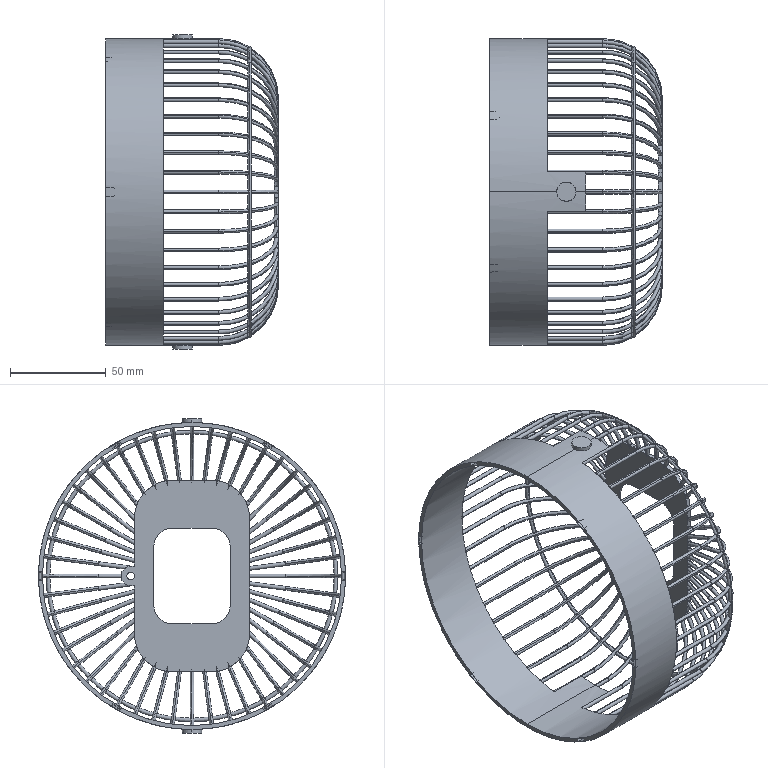Part | SolidWorks | features ICE 8, Revolution 3, MirrorSolid 2, CirPattern 1, CombineBodies 1, MirrorPattern 1, MoveCopyBody 1, Sweep 1 | 1 solid | 410 faces | box 90 x 160 x 164 mm | volume 49564 mm3 | cylinder 189 | plane 109 | torus 100 | cone 12 | commonest cylinder face diameters 2 x156 10 x10 40 x8 20 x4 36 x4 4 x2